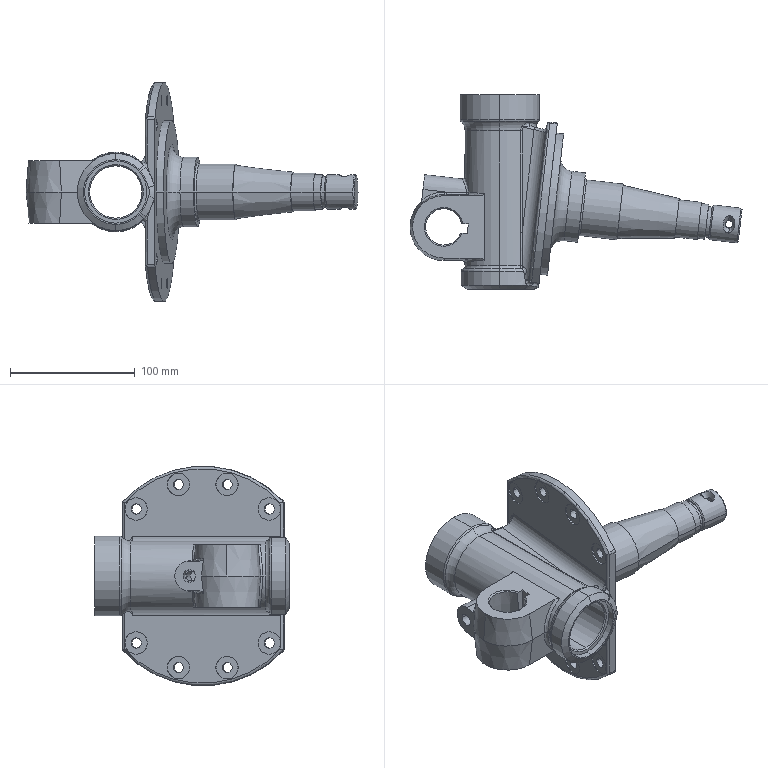Part | SolidWorks | features Chamfer 5, Fillet 4, HoleWzd 3, ICE 2, 3DProfileFeature 1, BaseBody 1, RevCut 1, Revolution 1, VarFillet 1 | 1 solid | 208 faces | box 266.225 x 156 x 176 mm | volume 686128 mm3 | cylinder 91 | plane 44 | spline 35 | torus 18 | cone 18 | sphere 2 | commonest cylinder face diameters 8.25 x16 18 x16 4 x11 56 x7 6 x6 28 x4